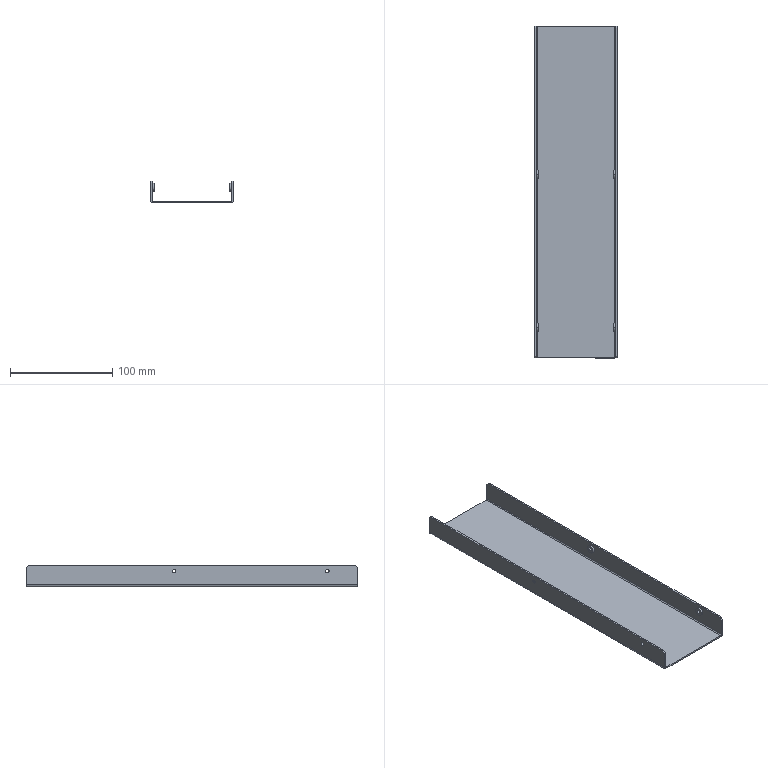Part | SolidWorks | features Chamfer 1, EdgeFlange 1, FlatPattern 1, HoleWzd 1, ICE 1, MirrorPattern 1, SMBaseFlange 1, SheetMetal 1 | 1 solid | 46 faces | box 81 x 325 x 21.5 mm | volume 58526 mm3 | plane 26 | cylinder 20 | commonest cylinder face diameters 3.3 x8 8 x8 2 x2 5 x2
STEP:
#1=CARTESIAN_POINT('',(37.,-132.5,12.35));
#2=VERTEX_POINT('',#1);
#3=CARTESIAN_POINT('',(37.,-132.5,15.65));
#4=VERTEX_POINT('',#3);
#5=CARTESIAN_POINT('',(37.,-132.5,14.));
#6=DIRECTION('',(-1.,0.,0.));
#7=DIRECTION('',(0.,0.,1.));
#8=AXIS2_PLACEMENT_3D('',#5,#6,#7);
#9=CIRCLE('',#8,1.65);
#10=EDGE_CURVE('',#2,#4,#9,.T.);
#11=ORIENTED_EDGE('',*,*,#10,.T.);
#12=CARTESIAN_POINT('',(40.5,-132.5,15.65));
#13=VERTEX_POINT('',#12);
#14=CARTESIAN_POINT('',(40.5,-132.5,15.65));
#15=DIRECTION('',(1.,0.,0.));
#16=VECTOR('',#15,1000.);
#17=LINE('',#14,#16);
#18=EDGE_CURVE('',#4,#13,#17,.T.);
#19=ORIENTED_EDGE('',*,*,#18,.T.);
#20=CARTESIAN_POINT('',(40.5,-132.5,12.35));
#21=VERTEX_POINT('',#20);
#22=CARTESIAN_POINT('',(40.5,-132.5,14.));
#23=DIRECTION('',(1.,0.,0.));
#24=DIRECTION('',(0.,0.,-1.));
#25=AXIS2_PLACEMENT_3D('',#22,#23,#24);
#26=CIRCLE('',#25,1.65);
#27=EDGE_CURVE('',#13,#21,#26,.T.);
#28=ORIENTED_EDGE('',*,*,#27,.T.);
#29=CARTESIAN_POINT('',(40.5,-132.5,12.35));
#30=DIRECTION('',(1.,0.,0.));
#31=VECTOR('',#30,1000.);
#32=LINE('',#29,#31);
#33=EDGE_CURVE('',#2,#21,#32,.T.);
#34=ORIENTED_EDGE('',*,*,#33,.F.);
#35=EDGE_LOOP('',(#11,#19,#28,#34));
#36=FACE_OUTER_BOUND('',#35,.T.);
#37=CARTESIAN_POINT('',(40.5,-132.5,14.));
#38=DIRECTION('',(1.,0.,0.));
#39=DIRECTION('',(0.,0.,-1.));
#40=AXIS2_PLACEMENT_3D('',#37,#38,#39);
#41=CYLINDRICAL_SURFACE('',#40,1.65);
#42=ADVANCED_FACE('',(#36),#41,.F.);
#43=CARTESIAN_POINT('',(37.,17.5,12.35));
#44=VERTEX_POINT('',#43);
#45=CARTESIAN_POINT('',(37.,17.5,15.65));
#46=VERTEX_POINT('',#45);
#47=CARTESIAN_POINT('',(37.,17.5,14.));
#48=DIRECTION('',(-1.,0.,0.));
#49=DIRECTION('',(0.,0.,1.));
#50=AXIS2_PLACEMENT_3D('',#47,#48,#49);
#51=CIRCLE('',#50,1.65);
#52=EDGE_CURVE('',#44,#46,#51,.T.);
#53=ORIENTED_EDGE('',*,*,#52,.T.);
#54=CARTESIAN_POINT('',(40.5,17.5,15.65));
#55=VERTEX_POINT('',#54);
#56=CARTESIAN_POINT('',(40.5,17.5,15.65));
#57=DIRECTION('',(1.,0.,0.));
#58=VECTOR('',#57,1000.);
#59=LINE('',#56,#58);
#60=EDGE_CURVE('',#46,#55,#59,.T.);
#61=ORIENTED_EDGE('',*,*,#60,.T.);
#62=CARTESIAN_POINT('',(40.5,17.5,12.35));
#63=VERTEX_POINT('',#62);
#64=CARTESIAN_POINT('',(40.5,17.5,14.));
#65=DIRECTION('',(1.,0.,0.));
#66=DIRECTION('',(0.,0.,-1.));
#67=AXIS2_PLACEMENT_3D('',#64,#65,#66);
#68=CIRCLE('',#67,1.65);
#69=EDGE_CURVE('',#55,#63,#68,.T.);
#70=ORIENTED_EDGE('',*,*,#69,.T.);
#71=CARTESIAN_POINT('',(40.5,17.5,12.35));
#72=DIRECTION('',(1.,0.,0.));
#73=VECTOR('',#72,1000.);
#74=LINE('',#71,#73);
#75=EDGE_CURVE('',#44,#63,#74,.T.);
#76=ORIENTED_EDGE('',*,*,#75,.F.);
#77=EDGE_LOOP('',(#53,#61,#70,#76));
#78=FACE_OUTER_BOUND('',#77,.T.);
#79=CARTESIAN_POINT('',(40.5,17.5,14.));
#80=DIRECTION('',(1.,0.,0.));
#81=DIRECTION('',(0.,0.,-1.));
#82=AXIS2_PLACEMENT_3D('',#79,#80,#81);
#83=CYLINDRICAL_SURFACE('',#82,1.65);
#84=ADVANCED_FACE('',(#78),#83,.F.);
#85=CARTESIAN_POINT('',(37.,-132.5,10.));
#86=VERTEX_POINT('',#85);
#87=CARTESIAN_POINT('',(37.,-132.5,18.));
#88=VERTEX_POINT('',#87);
#89=CARTESIAN_POINT('',(37.,-132.5,14.));
#90=DIRECTION('',(1.,0.,0.));
#91=DIRECTION('',(0.,0.,-1.));
#92=AXIS2_PLACEMENT_3D('',#89,#90,#91);
#93=CIRCLE('',#92,4.);
#94=EDGE_CURVE('',#86,#88,#93,.T.);
#95=ORIENTED_EDGE('',*,*,#94,.T.);
#96=CARTESIAN_POINT('',(39.,-132.5,18.));
#97=VERTEX_POINT('',#96);
#98=CARTESIAN_POINT('',(37.,-132.5,18.));
#99=DIRECTION('',(1.,0.,0.));
#100=VECTOR('',#99,1000.);
#101=LINE('',#98,#100);
#102=EDGE_CURVE('',#88,#97,#101,.T.);
#103=ORIENTED_EDGE('',*,*,#102,.T.);
#104=CARTESIAN_POINT('',(39.,-132.5,10.));
#105=VERTEX_POINT('',#104);
#106=CARTESIAN_POINT('',(39.,-132.5,14.));
#107=DIRECTION('',(-1.,0.,0.));
#108=DIRECTION('',(0.,0.,1.));
#109=AXIS2_PLACEMENT_3D('',#106,#107,#108);
#110=CIRCLE('',#109,4.);
#111=EDGE_CURVE('',#97,#105,#110,.T.);
#112=ORIENTED_EDGE('',*,*,#111,.T.);
#113=CARTESIAN_POINT('',(37.,-132.5,10.));
#114=DIRECTION('',(1.,0.,0.));
#115=VECTOR('',#114,1000.);
#116=LINE('',#113,#115);
#117=EDGE_CURVE('',#86,#105,#116,.T.);
#118=ORIENTED_EDGE('',*,*,#117,.F.);
#119=EDGE_LOOP('',(#95,#103,#112,#118));
#120=FACE_OUTER_BOUND('',#119,.T.);
#121=CARTESIAN_POINT('',(37.,-132.5,14.));
#122=DIRECTION('',(1.,0.,0.));
#123=DIRECTION('',(0.,0.,-1.));
#124=AXIS2_PLACEMENT_3D('',#121,#122,#123);
#125=CYLINDRICAL_SURFACE('',#124,4.);
#126=ADVANCED_FACE('',(#120),#125,.T.);
#127=CARTESIAN_POINT('',(37.,17.5,10.));
#128=VERTEX_POINT('',#127);
#129=CARTESIAN_POINT('',(37.,17.5,18.));
#130=VERTEX_POINT('',#129);
#131=CARTESIAN_POINT('',(37.,17.5,14.));
#132=DIRECTION('',(1.,0.,0.));
#133=DIRECTION('',(0.,0.,-1.));
#134=AXIS2_PLACEMENT_3D('',#131,#132,#133);
#135=CIRCLE('',#134,4.);
#136=EDGE_CURVE('',#128,#130,#135,.T.);
#137=ORIENTED_EDGE('',*,*,#136,.T.);
#138=CARTESIAN_POINT('',(39.,17.5,18.));
#139=VERTEX_POINT('',#138);
#140=CARTESIAN_POINT('',(37.,17.5,18.));
#141=DIRECTION('',(1.,0.,0.));
#142=VECTOR('',#141,1000.);
#143=LINE('',#140,#142);
#144=EDGE_CURVE('',#130,#139,#143,.T.);
#145=ORIENTED_EDGE('',*,*,#144,.T.);
#146=CARTESIAN_POINT('',(39.,17.5,10.));
#147=VERTEX_POINT('',#146);
#148=CARTESIAN_POINT('',(39.,17.5,14.));
#149=DIRECTION('',(-1.,0.,0.));
#150=DIRECTION('',(0.,0.,1.));
#151=AXIS2_PLACEMENT_3D('',#148,#149,#150);
#152=CIRCLE('',#151,4.);
#153=EDGE_CURVE('',#139,#147,#152,.T.);
#154=ORIENTED_EDGE('',*,*,#153,.T.);
#155=CARTESIAN_POINT('',(37.,17.5,10.));
#156=DIRECTION('',(1.,0.,0.));
#157=VECTOR('',#156,1000.);
#158=LINE('',#155,#157);
#159=EDGE_CURVE('',#128,#147,#158,.T.);
#160=ORIENTED_EDGE('',*,*,#159,.F.);
#161=EDGE_LOOP('',(#137,#145,#154,#160));
#162=FACE_OUTER_BOUND('',#161,.T.);
#163=CARTESIAN_POINT('',(37.,17.5,14.));
#164=DIRECTION('',(1.,0.,0.));
#165=DIRECTION('',(0.,0.,-1.));
#166=AXIS2_PLACEMENT_3D('',#163,#164,#165);
#167=CYLINDRICAL_SURFACE('',#166,4.);
#168=ADVANCED_FACE('',(#162),#167,.T.);
#169=CARTESIAN_POINT('',(-37.,-132.5,15.65));
#170=VERTEX_POINT('',#169);
#171=CARTESIAN_POINT('',(-37.,-132.5,12.35));
#172=VERTEX_POINT('',#171);
#173=CARTESIAN_POINT('',(-37.,-132.5,14.));
#174=DIRECTION('',(1.,0.,0.));
#175=DIRECTION('',(0.,0.,-1.));
#176=AXIS2_PLACEMENT_3D('',#173,#174,#175);
#177=CIRCLE('',#176,1.65);
#178=EDGE_CURVE('',#170,#172,#177,.T.);
#179=ORIENTED_EDGE('',*,*,#178,.T.);
#180=CARTESIAN_POINT('',(-40.5,-132.5,12.35));
#181=VERTEX_POINT('',#180);
#182=CARTESIAN_POINT('',(-40.5,-132.5,12.35));
#183=DIRECTION('',(-1.,0.,0.));
#184=VECTOR('',#183,1000.);
#185=LINE('',#182,#184);
#186=EDGE_CURVE('',#172,#181,#185,.T.);
#187=ORIENTED_EDGE('',*,*,#186,.T.);
#188=CARTESIAN_POINT('',(-40.5,-132.5,15.65));
#189=VERTEX_POINT('',#188);
#190=CARTESIAN_POINT('',(-40.5,-132.5,14.));
#191=DIRECTION('',(-1.,0.,0.));
#192=DIRECTION('',(0.,0.,1.));
#193=AXIS2_PLACEMENT_3D('',#190,#191,#192);
#194=CIRCLE('',#193,1.65);
#195=EDGE_CURVE('',#181,#189,#194,.T.);
#196=ORIENTED_EDGE('',*,*,#195,.T.);
#197=CARTESIAN_POINT('',(-40.5,-132.5,15.65));
#198=DIRECTION('',(-1.,0.,0.));
#199=VECTOR('',#198,1000.);
#200=LINE('',#197,#199);
#201=EDGE_CURVE('',#170,#189,#200,.T.);
#202=ORIENTED_EDGE('',*,*,#201,.F.);
#203=EDGE_LOOP('',(#179,#187,#196,#202));
#204=FACE_OUTER_BOUND('',#203,.T.);
#205=CARTESIAN_POINT('',(-40.5,-132.5,14.));
#206=DIRECTION('',(-1.,0.,0.));
#207=DIRECTION('',(0.,0.,1.));
#208=AXIS2_PLACEMENT_3D('',#205,#206,#207);
#209=CYLINDRICAL_SURFACE('',#208,1.65);
#210=ADVANCED_FACE('',(#204),#209,.F.);
#211=CARTESIAN_POINT('',(-37.,17.5,15.65));
#212=VERTEX_POINT('',#211);
#213=CARTESIAN_POINT('',(-37.,17.5,12.35));
#214=VERTEX_POINT('',#213);
#215=CARTESIAN_POINT('',(-37.,17.5,14.));
#216=DIRECTION('',(1.,0.,0.));
#217=DIRECTION('',(0.,0.,-1.));
#218=AXIS2_PLACEMENT_3D('',#215,#216,#217);
#219=CIRCLE('',#218,1.65);
#220=EDGE_CURVE('',#212,#214,#219,.T.);
#221=ORIENTED_EDGE('',*,*,#220,.T.);
#222=CARTESIAN_POINT('',(-40.5,17.5,12.35));
#223=VERTEX_POINT('',#222);
#224=CARTESIAN_POINT('',(-40.5,17.5,12.35));
#225=DIRECTION('',(-1.,0.,0.));
#226=VECTOR('',#225,1000.);
#227=LINE('',#224,#226);
#228=EDGE_CURVE('',#214,#223,#227,.T.);
#229=ORIENTED_EDGE('',*,*,#228,.T.);
#230=CARTESIAN_POINT('',(-40.5,17.5,15.65));
#231=VERTEX_POINT('',#230);
#232=CARTESIAN_POINT('',(-40.5,17.5,14.));
#233=DIRECTION('',(-1.,0.,0.));
#234=DIRECTION('',(0.,0.,1.));
#235=AXIS2_PLACEMENT_3D('',#232,#233,#234);
#236=CIRCLE('',#235,1.65);
#237=EDGE_CURVE('',#223,#231,#236,.T.);
#238=ORIENTED_EDGE('',*,*,#237,.T.);
#239=CARTESIAN_POINT('',(-40.5,17.5,15.65));
#240=DIRECTION('',(-1.,0.,0.));
#241=VECTOR('',#240,1000.);
#242=LINE('',#239,#241);
#243=EDGE_CURVE('',#212,#231,#242,.T.);
#244=ORIENTED_EDGE('',*,*,#243,.F.);
#245=EDGE_LOOP('',(#221,#229,#238,#244));
#246=FACE_OUTER_BOUND('',#245,.T.);
#247=CARTESIAN_POINT('',(-40.5,17.5,14.));
#248=DIRECTION('',(-1.,0.,0.));
#249=DIRECTION('',(0.,0.,1.));
#250=AXIS2_PLACEMENT_3D('',#247,#248,#249);
#251=CYLINDRICAL_SURFACE('',#250,1.65);
#252=ADVANCED_FACE('',(#246),#251,.F.);
#253=CARTESIAN_POINT('',(-37.,-132.5,10.));
#254=VERTEX_POINT('',#253);
#255=CARTESIAN_POINT('',(-37.,-132.5,18.));
#256=VERTEX_POINT('',#255);
#257=CARTESIAN_POINT('',(-37.,-132.5,14.));
#258=DIRECTION('',(1.,0.,0.));
#259=DIRECTION('',(0.,0.,-1.));
#260=AXIS2_PLACEMENT_3D('',#257,#258,#259);
#261=CIRCLE('',#260,4.);
#262=EDGE_CURVE('',#254,#256,#261,.T.);
#263=ORIENTED_EDGE('',*,*,#262,.F.);
#264=CARTESIAN_POINT('',(-39.,-132.5,10.));
#265=VERTEX_POINT('',#264);
#266=CARTESIAN_POINT('',(-37.,-132.5,10.));
#267=DIRECTION('',(-1.,0.,0.));
#268=VECTOR('',#267,1000.);
#269=LINE('',#266,#268);
#270=EDGE_CURVE('',#254,#265,#269,.T.);
#271=ORIENTED_EDGE('',*,*,#270,.T.);
#272=CARTESIAN_POINT('',(-39.,-132.5,18.));
#273=VERTEX_POINT('',#272);
#274=CARTESIAN_POINT('',(-39.,-132.5,14.));
#275=DIRECTION('',(1.,0.,0.));
#276=DIRECTION('',(0.,0.,-1.));
#277=AXIS2_PLACEMENT_3D('',#274,#275,#276);
#278=CIRCLE('',#277,4.);
#279=EDGE_CURVE('',#265,#273,#278,.T.);
#280=ORIENTED_EDGE('',*,*,#279,.T.);
#281=CARTESIAN_POINT('',(-37.,-132.5,18.));
#282=DIRECTION('',(-1.,0.,0.));
#283=VECTOR('',#282,1000.);
#284=LINE('',#281,#283);
#285=EDGE_CURVE('',#256,#273,#284,.T.);
#286=ORIENTED_EDGE('',*,*,#285,.F.);
#287=EDGE_LOOP('',(#263,#271,#280,#286));
#288=FACE_OUTER_BOUND('',#287,.T.);
#289=CARTESIAN_POINT('',(-37.,-132.5,14.));
#290=DIRECTION('',(-1.,0.,0.));
#291=DIRECTION('',(0.,0.,1.));
#292=AXIS2_PLACEMENT_3D('',#289,#290,#291);
#293=CYLINDRICAL_SURFACE('',#292,4.);
#294=ADVANCED_FACE('',(#288),#293,.T.);
#295=CARTESIAN_POINT('',(-37.,17.5,10.));
#296=VERTEX_POINT('',#295);
#297=CARTESIAN_POINT('',(-37.,17.5,18.));
#298=VERTEX_POINT('',#297);
#299=CARTESIAN_POINT('',(-37.,17.5,14.));
#300=DIRECTION('',(1.,0.,0.));
#301=DIRECTION('',(0.,0.,-1.));
#302=AXIS2_PLACEMENT_3D('',#299,#300,#301);
#303=CIRCLE('',#302,4.);
#304=EDGE_CURVE('',#296,#298,#303,.T.);
#305=ORIENTED_EDGE('',*,*,#304,.F.);
#306=CARTESIAN_POINT('',(-39.,17.5,10.));
#307=VERTEX_POINT('',#306);
#308=CARTESIAN_POINT('',(-37.,17.5,10.));
#309=DIRECTION('',(-1.,0.,0.));
#310=VECTOR('',#309,1000.);
#311=LINE('',#308,#310);
#312=EDGE_CURVE('',#296,#307,#311,.T.);
#313=ORIENTED_EDGE('',*,*,#312,.T.);
#314=CARTESIAN_POINT('',(-39.,17.5,18.));
#315=VERTEX_POINT('',#314);
#316=CARTESIAN_POINT('',(-39.,17.5,14.));
#317=DIRECTION('',(1.,0.,0.));
#318=DIRECTION('',(0.,0.,-1.));
#319=AXIS2_PLACEMENT_3D('',#316,#317,#318);
#320=CIRCLE('',#319,4.);
#321=EDGE_CURVE('',#307,#315,#320,.T.);
#322=ORIENTED_EDGE('',*,*,#321,.T.);
#323=CARTESIAN_POINT('',(-37.,17.5,18.));
#324=DIRECTION('',(-1.,0.,0.));
#325=VECTOR('',#324,1000.);
#326=LINE('',#323,#325);
#327=EDGE_CURVE('',#298,#315,#326,.T.);
#328=ORIENTED_EDGE('',*,*,#327,.F.);
#329=EDGE_LOOP('',(#305,#313,#322,#328));
#330=FACE_OUTER_BOUND('',#329,.T.);
#331=CARTESIAN_POINT('',(-37.,17.5,14.));
#332=DIRECTION('',(-1.,0.,0.));
#333=DIRECTION('',(0.,0.,1.));
#334=AXIS2_PLACEMENT_3D('',#331,#332,#333);
#335=CYLINDRICAL_SURFACE('',#334,4.);
#336=ADVANCED_FACE('',(#330),#335,.T.);
#337=CARTESIAN_POINT('',(40.5,160.5,20.));
#338=VERTEX_POINT('',#337);
#339=CARTESIAN_POINT('',(40.5,-160.5,20.));
#340=VERTEX_POINT('',#339);
#341=CARTESIAN_POINT('',(40.5,-162.5,20.));
#342=DIRECTION('',(0.,-1.,0.));
#343=VECTOR('',#342,1000.);
#344=LINE('',#341,#343);
#345=EDGE_CURVE('',#338,#340,#344,.T.);
#346=ORIENTED_EDGE('',*,*,#345,.T.);
#347=CARTESIAN_POINT('',(40.5,-162.5,18.));
#348=VERTEX_POINT('',#347);
#349=CARTESIAN_POINT('',(40.5,-162.5,18.));
#350=DIRECTION('',(0.,-0.7071,-0.7071));
#351=VECTOR('',#350,1000.);
#352=LINE('',#349,#351);
#353=EDGE_CURVE('',#340,#348,#352,.T.);
#354=ORIENTED_EDGE('',*,*,#353,.T.);
#355=CARTESIAN_POINT('',(40.5,-162.5,1.));
#356=VERTEX_POINT('',#355);
#357=CARTESIAN_POINT('',(40.5,-162.5,0.));
#358=DIRECTION('',(0.,0.,-1.));
#359=VECTOR('',#358,1000.);
#360=LINE('',#357,#359);
#361=EDGE_CURVE('',#348,#356,#360,.T.);
#362=ORIENTED_EDGE('',*,*,#361,.T.);
#363=CARTESIAN_POINT('',(40.5,162.5,1.));
#364=VERTEX_POINT('',#363);
#365=CARTESIAN_POINT('',(40.5,0.,1.));
#366=DIRECTION('',(0.,-1.,0.));
#367=VECTOR('',#366,1000.);
#368=LINE('',#365,#367);
#369=EDGE_CURVE('',#364,#356,#368,.T.);
#370=ORIENTED_EDGE('',*,*,#369,.F.);
#371=CARTESIAN_POINT('',(40.5,162.5,18.));
#372=VERTEX_POINT('',#371);
#373=CARTESIAN_POINT('',(40.5,162.5,20.));
#374=DIRECTION('',(0.,0.,1.));
#375=VECTOR('',#374,1000.);
#376=LINE('',#373,#375);
#377=EDGE_CURVE('',#364,#372,#376,.T.);
#378=ORIENTED_EDGE('',*,*,#377,.T.);
#379=CARTESIAN_POINT('',(40.5,160.5,20.));
#380=DIRECTION('',(0.,-0.7071,0.7071));
#381=VECTOR('',#380,1000.);
#382=LINE('',#379,#381);
#383=EDGE_CURVE('',#372,#338,#382,.T.);
#384=ORIENTED_EDGE('',*,*,#383,.T.);
#385=EDGE_LOOP('',(#346,#354,#362,#370,#378,#384));
#386=FACE_OUTER_BOUND('',#385,.T.);
#387=CARTESIAN_POINT('',(40.5,17.5,14.));
#388=DIRECTION('',(1.,0.,0.));
#389=DIRECTION('',(0.,0.,-1.));
#390=AXIS2_PLACEMENT_3D('',#387,#388,#389);
#391=CIRCLE('',#390,1.65);
#392=EDGE_CURVE('',#63,#55,#391,.T.);
#393=ORIENTED_EDGE('',*,*,#392,.F.);
#394=ORIENTED_EDGE('',*,*,#69,.F.);
#395=EDGE_LOOP('',(#393,#394));
#396=FACE_BOUND('',#395,.T.);
#397=CARTESIAN_POINT('',(40.5,-132.5,14.));
#398=DIRECTION('',(1.,0.,0.));
#399=DIRECTION('',(0.,0.,-1.));
#400=AXIS2_PLACEMENT_3D('',#397,#398,#399);
#401=CIRCLE('',#400,1.65);
#402=EDGE_CURVE('',#21,#13,#401,.T.);
#403=ORIENTED_EDGE('',*,*,#402,.F.);
#404=ORIENTED_EDGE('',*,*,#27,.F.);
#405=EDGE_LOOP('',(#403,#404));
#406=FACE_BOUND('',#405,.T.);
#407=CARTESIAN_POINT('',(40.5,0.,0.));
#408=DIRECTION('',(-1.,0.,0.));
#409=DIRECTION('',(0.,0.,1.));
#410=AXIS2_PLACEMENT_3D('',#407,#408,#409);
#411=PLANE('',#410);
#412=ADVANCED_FACE('',(#386,#396,#406),#411,.F.);
#413=CARTESIAN_POINT('',(-39.,17.5,14.));
#414=DIRECTION('',(1.,0.,0.));
#415=DIRECTION('',(0.,0.,-1.));
#416=AXIS2_PLACEMENT_3D('',#413,#414,#415);
#417=CIRCLE('',#416,4.);
#418=EDGE_CURVE('',#315,#307,#417,.T.);
#419=ORIENTED_EDGE('',*,*,#418,.F.);
#420=ORIENTED_EDGE('',*,*,#321,.F.);
#421=EDGE_LOOP('',(#419,#420));
#422=FACE_BOUND('',#421,.T.);
#423=CARTESIAN_POINT('',(-39.,-160.5,20.));
#424=VERTEX_POINT('',#423);
#425=CARTESIAN_POINT('',(-39.,160.5,20.));
#426=VERTEX_POINT('',#425);
#427=CARTESIAN_POINT('',(-39.,162.5,20.));
#428=DIRECTION('',(0.,1.,0.));
#429=VECTOR('',#428,1000.);
#430=LINE('',#427,#429);
#431=EDGE_CURVE('',#424,#426,#430,.T.);
#432=ORIENTED_EDGE('',*,*,#431,.F.);
#433=CARTESIAN_POINT('',(-39.,-162.5,18.));
#434=VERTEX_POINT('',#433);
#435=CARTESIAN_POINT('',(-39.,-90.25,90.25));
#436=DIRECTION('',(0.,-0.7071,-0.7071));
#437=VECTOR('',#436,1000.);
#438=LINE('',#435,#437);
#439=EDGE_CURVE('',#424,#434,#438,.T.);
#440=ORIENTED_EDGE('',*,*,#439,.T.);
#441=CARTESIAN_POINT('',(-39.,-162.5,1.));
#442=VERTEX_POINT('',#441);
#443=CARTESIAN_POINT('',(-39.,-162.5,20.));
#444=DIRECTION('',(0.,0.,1.));
#445=VECTOR('',#444,1000.);
#446=LINE('',#443,#445);
#447=EDGE_CURVE('',#442,#434,#446,.T.);
#448=ORIENTED_EDGE('',*,*,#447,.F.);
#449=CARTESIAN_POINT('',(-39.,162.5,1.));
#450=VERTEX_POINT('',#449);
#451=CARTESIAN_POINT('',(-39.,162.5,1.));
#452=DIRECTION('',(0.,-1.,0.));
#453=VECTOR('',#452,1000.);
#454=LINE('',#451,#453);
#455=EDGE_CURVE('',#450,#442,#454,.T.);
#456=ORIENTED_EDGE('',*,*,#455,.F.);
#457=CARTESIAN_POINT('',(-39.,162.5,18.));
#458=VERTEX_POINT('',#457);
#459=CARTESIAN_POINT('',(-39.,162.5,0.));
#460=DIRECTION('',(0.,0.,-1.));
#461=VECTOR('',#460,1000.);
#462=LINE('',#459,#461);
#463=EDGE_CURVE('',#458,#450,#462,.T.);
#464=ORIENTED_EDGE('',*,*,#463,.F.);
#465=CARTESIAN_POINT('',(-39.,90.25,90.25));
#466=DIRECTION('',(0.,-0.7071,0.7071));
#467=VECTOR('',#466,1000.);
#468=LINE('',#465,#467);
#469=EDGE_CURVE('',#458,#426,#468,.T.);
#470=ORIENTED_EDGE('',*,*,#469,.T.);
#471=EDGE_LOOP('',(#432,#440,#448,#456,#464,#470));
#472=FACE_OUTER_BOUND('',#471,.T.);
#473=CARTESIAN_POINT('',(-39.,-132.5,14.));
#474=DIRECTION('',(1.,0.,0.));
#475=DIRECTION('',(0.,0.,-1.));
#476=AXIS2_PLACEMENT_3D('',#473,#474,#475);
#477=CIRCLE('',#476,4.);
#478=EDGE_CURVE('',#273,#265,#477,.T.);
#479=ORIENTED_EDGE('',*,*,#478,.F.);
#480=ORIENTED_EDGE('',*,*,#279,.F.);
#481=EDGE_LOOP('',(#479,#480));
#482=FACE_BOUND('',#481,.T.);
#483=CARTESIAN_POINT('',(-39.,0.,0.));
#484=DIRECTION('',(1.,0.,0.));
#485=DIRECTION('',(0.,0.,-1.));
#486=AXIS2_PLACEMENT_3D('',#483,#484,#485);
#487=PLANE('',#486);
#488=ADVANCED_FACE('',(#422,#472,#482),#487,.T.);
#489=CARTESIAN_POINT('',(38.,162.5,-1.5));
#490=VERTEX_POINT('',#489);
#491=CARTESIAN_POINT('',(38.,-162.5,-1.5));
#492=VERTEX_POINT('',#491);
#493=CARTESIAN_POINT('',(38.,162.5,-1.5));
#494=DIRECTION('',(0.,-1.,0.));
#495=VECTOR('',#494,1000.);
#496=LINE('',#493,#495);
#497=EDGE_CURVE('',#490,#492,#496,.T.);
#498=ORIENTED_EDGE('',*,*,#497,.T.);
#499=CARTESIAN_POINT('',(-38.,-162.5,-1.5));
#500=VERTEX_POINT('',#499);
#501=CARTESIAN_POINT('',(-39.,-162.5,-1.5));
#502=DIRECTION('',(1.,0.,0.));
#503=VECTOR('',#502,1000.);
#504=LINE('',#501,#503);
#505=EDGE_CURVE('',#500,#492,#504,.T.);
#506=ORIENTED_EDGE('',*,*,#505,.F.);
#507=CARTESIAN_POINT('',(-38.,162.5,-1.5));
#508=VERTEX_POINT('',#507);
#509=CARTESIAN_POINT('',(-38.,-162.5,-1.5));
#510=DIRECTION('',(0.,1.,0.));
#511=VECTOR('',#510,1000.);
#512=LINE('',#509,#511);
#513=EDGE_CURVE('',#500,#508,#512,.T.);
#514=ORIENTED_EDGE('',*,*,#513,.T.);
#515=CARTESIAN_POINT('',(-39.,162.5,-1.5));
#516=DIRECTION('',(-1.,0.,0.));
#517=VECTOR('',#516,1000.);
#518=LINE('',#515,#517);
#519=EDGE_CURVE('',#490,#508,#518,.T.);
#520=ORIENTED_EDGE('',*,*,#519,.F.);
#521=EDGE_LOOP('',(#498,#506,#514,#520));
#522=FACE_OUTER_BOUND('',#521,.T.);
#523=CARTESIAN_POINT('',(0.,0.,-1.5));
#524=DIRECTION('',(0.,0.,1.));
#525=DIRECTION('',(1.,0.,0.));
#526=AXIS2_PLACEMENT_3D('',#523,#524,#525);
#527=PLANE('',#526);
#528=ADVANCED_FACE('',(#522),#527,.F.);
#529=CARTESIAN_POINT('',(-38.,-162.5,0.));
#530=VERTEX_POINT('',#529);
#531=CARTESIAN_POINT('',(38.,-162.5,0.));
#532=VERTEX_POINT('',#531);
#533=CARTESIAN_POINT('',(-39.,-162.5,0.));
#534=DIRECTION('',(1.,0.,0.));
#535=VECTOR('',#534,1000.);
#536=LINE('',#533,#535);
#537=EDGE_CURVE('',#530,#532,#536,.T.);
#538=ORIENTED_EDGE('',*,*,#537,.T.);
#539=CARTESIAN_POINT('',(38.,162.5,0.));
#540=VERTEX_POINT('',#539);
#541=CARTESIAN_POINT('',(38.,162.5,0.));
#542=DIRECTION('',(0.,-1.,0.));
#543=VECTOR('',#542,1000.);
#544=LINE('',#541,#543);
#545=EDGE_CURVE('',#540,#532,#544,.T.);
#546=ORIENTED_EDGE('',*,*,#545,.F.);
#547=CARTESIAN_POINT('',(-38.,162.5,0.));
#548=VERTEX_POINT('',#547);
#549=CARTESIAN_POINT('',(-39.,162.5,0.));
#550=DIRECTION('',(-1.,0.,0.));
#551=VECTOR('',#550,1000.);
#552=LINE('',#549,#551);
#553=EDGE_CURVE('',#540,#548,#552,.T.);
#554=ORIENTED_EDGE('',*,*,#553,.T.);
#555=CARTESIAN_POINT('',(-38.,-162.5,0.));
#556=DIRECTION('',(0.,1.,0.));
#557=VECTOR('',#556,1000.);
#558=LINE('',#555,#557);
#559=EDGE_CURVE('',#530,#548,#558,.T.);
#560=ORIENTED_EDGE('',*,*,#559,.F.);
#561=EDGE_LOOP('',(#538,#546,#554,#560));
#562=FACE_OUTER_BOUND('',#561,.T.);
#563=CARTESIAN_POINT('',(0.,0.,0.));
#564=DIRECTION('',(0.,0.,1.));
#565=DIRECTION('',(1.,0.,0.));
#566=AXIS2_PLACEMENT_3D('',#563,#564,#565);
#567=PLANE('',#566);
#568=ADVANCED_FACE('',(#562),#567,.T.);
#569=ORIENTED_EDGE('',*,*,#553,.F.);
#570=CARTESIAN_POINT('',(38.,162.5,0.));
#571=DIRECTION('',(0.,0.,-1.));
#572=VECTOR('',#571,1000.);
#573=LINE('',#570,#572);
#574=EDGE_CURVE('',#540,#490,#573,.T.);
#575=ORIENTED_EDGE('',*,*,#574,.T.);
#576=ORIENTED_EDGE('',*,*,#519,.T.);
#577=CARTESIAN_POINT('',(-38.,162.5,0.));
#578=DIRECTION('',(0.,0.,-1.));
#579=VECTOR('',#578,1000.);
#580=LINE('',#577,#579);
#581=EDGE_CURVE('',#548,#508,#580,.T.);
#582=ORIENTED_EDGE('',*,*,#581,.F.);
#583=EDGE_LOOP('',(#569,#575,#576,#582));
#584=FACE_OUTER_BOUND('',#583,.T.);
#585=CARTESIAN_POINT('',(-39.,162.5,-1.5));
#586=DIRECTION('',(0.,1.,0.));
#587=DIRECTION('',(0.,0.,1.));
#588=AXIS2_PLACEMENT_3D('',#585,#586,#587);
#589=PLANE('',#588);
#590=ADVANCED_FACE('',(#584),#589,.T.);
#591=CARTESIAN_POINT('',(38.,-162.5,0.));
#592=DIRECTION('',(0.,0.,-1.));
#593=VECTOR('',#592,1000.);
#594=LINE('',#591,#593);
#595=EDGE_CURVE('',#532,#492,#594,.T.);
#596=ORIENTED_EDGE('',*,*,#595,.F.);
#597=ORIENTED_EDGE('',*,*,#537,.F.);
#598=CARTESIAN_POINT('',(-38.,-162.5,0.));
#599=DIRECTION('',(0.,0.,-1.));
#600=VECTOR('',#599,1000.);
#601=LINE('',#598,#600);
#602=EDGE_CURVE('',#530,#500,#601,.T.);
#603=ORIENTED_EDGE('',*,*,#602,.T.);
#604=ORIENTED_EDGE('',*,*,#505,.T.);
#605=EDGE_LOOP('',(#596,#597,#603,#604));
#606=FACE_OUTER_BOUND('',#605,.T.);
#607=CARTESIAN_POINT('',(-39.,-162.5,-1.5));
#608=DIRECTION('',(0.,-1.,0.));
#609=DIRECTION('',(0.,0.,-1.));
#610=AXIS2_PLACEMENT_3D('',#607,#608,#609);
#611=PLANE('',#610);
#612=ADVANCED_FACE('',(#606),#611,.T.);
#613=CARTESIAN_POINT('',(-40.5,162.5,1.));
#614=VERTEX_POINT('',#613);
#615=CARTESIAN_POINT('',(-39.,162.5,1.));
#616=DIRECTION('',(-1.,0.,0.));
#617=VECTOR('',#616,1000.);
#618=LINE('',#615,#617);
#619=EDGE_CURVE('',#450,#614,#618,.T.);
#620=ORIENTED_EDGE('',*,*,#619,.F.);
#621=CARTESIAN_POINT('',(-38.,162.5,1.));
#622=DIRECTION('',(0.,1.,0.));
#623=DIRECTION('',(0.,0.,-1.));
#624=AXIS2_PLACEMENT_3D('',#621,#622,#623);
#625=CIRCLE('',#624,1.);
#626=EDGE_CURVE('',#548,#450,#625,.T.);
#627=ORIENTED_EDGE('',*,*,#626,.F.);
#628=ORIENTED_EDGE('',*,*,#581,.T.);
#629=CARTESIAN_POINT('',(-38.,162.5,1.));
#630=DIRECTION('',(0.,1.,0.));
#631=DIRECTION('',(0.,0.,-1.));
#632=AXIS2_PLACEMENT_3D('',#629,#630,#631);
#633=CIRCLE('',#632,2.5);
#634=EDGE_CURVE('',#508,#614,#633,.T.);
#635=ORIENTED_EDGE('',*,*,#634,.T.);
#636=EDGE_LOOP('',(#620,#627,#628,#635));
#637=FACE_OUTER_BOUND('',#636,.T.);
#638=CARTESIAN_POINT('',(-38.,162.5,1.));
#639=DIRECTION('',(0.,1.,0.));
#640=DIRECTION('',(0.,0.,1.));
#641=AXIS2_PLACEMENT_3D('',#638,#639,#640);
#642=PLANE('',#641);
#643=ADVANCED_FACE('',(#637),#642,.T.);
#644=CARTESIAN_POINT('',(-38.,-162.5,1.));
#645=DIRECTION('',(0.,-1.,0.));
#646=DIRECTION('',(0.,0.,-1.));
#647=AXIS2_PLACEMENT_3D('',#644,#645,#646);
#648=CIRCLE('',#647,1.);
#649=EDGE_CURVE('',#442,#530,#648,.T.);
#650=ORIENTED_EDGE('',*,*,#649,.F.);
#651=CARTESIAN_POINT('',(-40.5,-162.5,1.));
#652=VERTEX_POINT('',#651);
#653=CARTESIAN_POINT('',(-39.,-162.5,1.));
#654=DIRECTION('',(-1.,0.,0.));
#655=VECTOR('',#654,1000.);
#656=LINE('',#653,#655);
#657=EDGE_CURVE('',#442,#652,#656,.T.);
#658=ORIENTED_EDGE('',*,*,#657,.T.);
#659=CARTESIAN_POINT('',(-38.,-162.5,1.));
#660=DIRECTION('',(0.,-1.,0.));
#661=DIRECTION('',(0.,0.,-1.));
#662=AXIS2_PLACEMENT_3D('',#659,#660,#661);
#663=CIRCLE('',#662,2.5);
#664=EDGE_CURVE('',#652,#500,#663,.T.);
#665=ORIENTED_EDGE('',*,*,#664,.T.);
#666=ORIENTED_EDGE('',*,*,#602,.F.);
#667=EDGE_LOOP('',(#650,#658,#665,#666));
#668=FACE_OUTER_BOUND('',#667,.T.);
#669=CARTESIAN_POINT('',(-38.,-162.5,1.));
#670=DIRECTION('',(0.,1.,0.));
#671=DIRECTION('',(0.,0.,1.));
#672=AXIS2_PLACEMENT_3D('',#669,#670,#671);
#673=PLANE('',#672);
#674=ADVANCED_FACE('',(#668),#673,.F.);
#675=ORIENTED_EDGE('',*,*,#513,.F.);
#676=ORIENTED_EDGE('',*,*,#664,.F.);
#677=CARTESIAN_POINT('',(-40.5,0.,1.));
#678=DIRECTION('',(0.,1.,0.));
#679=VECTOR('',#678,1000.);
#680=LINE('',#677,#679);
#681=EDGE_CURVE('',#652,#614,#680,.T.);
#682=ORIENTED_EDGE('',*,*,#681,.T.);
#683=ORIENTED_EDGE('',*,*,#634,.F.);
#684=EDGE_LOOP('',(#675,#676,#682,#683));
#685=FACE_OUTER_BOUND('',#684,.T.);
#686=CARTESIAN_POINT('',(-38.,-162.5,1.));
#687=DIRECTION('',(0.,-1.,0.));
#688=DIRECTION('',(-1.,0.,0.));
#689=AXIS2_PLACEMENT_3D('',#686,#687,#688);
#690=CYLINDRICAL_SURFACE('',#689,2.5);
#691=ADVANCED_FACE('',(#685),#690,.T.);
#692=ORIENTED_EDGE('',*,*,#559,.T.);
#693=ORIENTED_EDGE('',*,*,#626,.T.);
#694=ORIENTED_EDGE('',*,*,#455,.T.);
#695=ORIENTED_EDGE('',*,*,#649,.T.);
#696=EDGE_LOOP('',(#692,#693,#694,#695));
#697=FACE_OUTER_BOUND('',#696,.T.);
#698=CARTESIAN_POINT('',(-38.,-162.5,1.));
#699=DIRECTION('',(0.,-1.,0.));
#700=DIRECTION('',(-1.,0.,0.));
#701=AXIS2_PLACEMENT_3D('',#698,#699,#700);
#702=CYLINDRICAL_SURFACE('',#701,1.);
#703=ADVANCED_FACE('',(#697),#702,.F.);
#704=ORIENTED_EDGE('',*,*,#447,.T.);
#705=CARTESIAN_POINT('',(-40.5,-162.5,18.));
#706=VERTEX_POINT('',#705);
#707=CARTESIAN_POINT('',(-40.5,-162.5,18.));
#708=DIRECTION('',(-1.,0.,0.));
#709=VECTOR('',#708,1000.);
#710=LINE('',#707,#709);
#711=EDGE_CURVE('',#434,#706,#710,.T.);
#712=ORIENTED_EDGE('',*,*,#711,.T.);
#713=CARTESIAN_POINT('',(-40.5,-162.5,20.));
#714=DIRECTION('',(0.,0.,1.));
#715=VECTOR('',#714,1000.);
#716=LINE('',#713,#715);
#717=EDGE_CURVE('',#652,#706,#716,.T.);
#718=ORIENTED_EDGE('',*,*,#717,.F.);
#719=ORIENTED_EDGE('',*,*,#657,.F.);
#720=EDGE_LOOP('',(#704,#712,#718,#719));
#721=FACE_OUTER_BOUND('',#720,.T.);
#722=CARTESIAN_POINT('',(-40.5,-162.5,20.));
#723=DIRECTION('',(0.,1.,0.));
#724=DIRECTION('',(-1.,0.,0.));
#725=AXIS2_PLACEMENT_3D('',#722,#723,#724);
#726=PLANE('',#725);
#727=ADVANCED_FACE('',(#721),#726,.F.);
#728=CARTESIAN_POINT('',(-40.5,162.5,18.));
#729=VERTEX_POINT('',#728);
#730=CARTESIAN_POINT('',(-40.5,162.5,0.));
#731=DIRECTION('',(0.,0.,-1.));
#732=VECTOR('',#731,1000.);
#733=LINE('',#730,#732);
#734=EDGE_CURVE('',#729,#614,#733,.T.);
#735=ORIENTED_EDGE('',*,*,#734,.F.);
#736=CARTESIAN_POINT('',(-40.5,162.5,18.));
#737=DIRECTION('',(1.,0.,0.));
#738=VECTOR('',#737,1000.);
#739=LINE('',#736,#738);
#740=EDGE_CURVE('',#729,#458,#739,.T.);
#741=ORIENTED_EDGE('',*,*,#740,.T.);
#742=ORIENTED_EDGE('',*,*,#463,.T.);
#743=ORIENTED_EDGE('',*,*,#619,.T.);
#744=EDGE_LOOP('',(#735,#741,#742,#743));
#745=FACE_OUTER_BOUND('',#744,.T.);
#746=CARTESIAN_POINT('',(-40.5,162.5,0.));
#747=DIRECTION('',(0.,-1.,0.));
#748=DIRECTION('',(1.,0.,0.));
#749=AXIS2_PLACEMENT_3D('',#746,#747,#748);
#750=PLANE('',#749);
#751=ADVANCED_FACE('',(#745),#750,.F.);
#752=CARTESIAN_POINT('',(-40.5,-132.5,14.));
#753=DIRECTION('',(-1.,0.,0.));
#754=DIRECTION('',(0.,0.,1.));
#755=AXIS2_PLACEMENT_3D('',#752,#753,#754);
#756=CIRCLE('',#755,1.65);
#757=EDGE_CURVE('',#189,#181,#756,.T.);
#758=ORIENTED_EDGE('',*,*,#757,.F.);
#759=ORIENTED_EDGE('',*,*,#195,.F.);
#760=EDGE_LOOP('',(#758,#759));
#761=FACE_BOUND('',#760,.T.);
#762=CARTESIAN_POINT('',(-40.5,17.5,14.));
#763=DIRECTION('',(-1.,0.,0.));
#764=DIRECTION('',(0.,0.,1.));
#765=AXIS2_PLACEMENT_3D('',#762,#763,#764);
#766=CIRCLE('',#765,1.65);
#767=EDGE_CURVE('',#231,#223,#766,.T.);
#768=ORIENTED_EDGE('',*,*,#767,.F.);
#769=ORIENTED_EDGE('',*,*,#237,.F.);
#770=EDGE_LOOP('',(#768,#769));
#771=FACE_BOUND('',#770,.T.);
#772=ORIENTED_EDGE('',*,*,#717,.T.);
#773=CARTESIAN_POINT('',(-40.5,-160.5,20.));
#774=VERTEX_POINT('',#773);
#775=CARTESIAN_POINT('',(-40.5,-160.5,20.));
#776=DIRECTION('',(0.,0.7071,0.7071));
#777=VECTOR('',#776,1000.);
#778=LINE('',#775,#777);
#779=EDGE_CURVE('',#706,#774,#778,.T.);
#780=ORIENTED_EDGE('',*,*,#779,.T.);
#781=CARTESIAN_POINT('',(-40.5,160.5,20.));
#782=VERTEX_POINT('',#781);
#783=CARTESIAN_POINT('',(-40.5,162.5,20.));
#784=DIRECTION('',(0.,1.,0.));
#785=VECTOR('',#784,1000.);
#786=LINE('',#783,#785);
#787=EDGE_CURVE('',#774,#782,#786,.T.);
#788=ORIENTED_EDGE('',*,*,#787,.T.);
#789=CARTESIAN_POINT('',(-40.5,162.5,18.));
#790=DIRECTION('',(0.,0.7071,-0.7071));
#791=VECTOR('',#790,1000.);
#792=LINE('',#789,#791);
#793=EDGE_CURVE('',#782,#729,#792,.T.);
#794=ORIENTED_EDGE('',*,*,#793,.T.);
#795=ORIENTED_EDGE('',*,*,#734,.T.);
#796=ORIENTED_EDGE('',*,*,#681,.F.);
#797=EDGE_LOOP('',(#772,#780,#788,#794,#795,#796));
#798=FACE_OUTER_BOUND('',#797,.T.);
#799=CARTESIAN_POINT('',(-40.5,0.,0.));
#800=DIRECTION('',(1.,0.,0.));
#801=DIRECTION('',(0.,0.,-1.));
#802=AXIS2_PLACEMENT_3D('',#799,#800,#801);
#803=PLANE('',#802);
#804=ADVANCED_FACE('',(#761,#771,#798),#803,.F.);
#805=ORIENTED_EDGE('',*,*,#787,.F.);
#806=CARTESIAN_POINT('',(-40.5,-160.5,20.));
#807=DIRECTION('',(1.,0.,0.));
#808=VECTOR('',#807,1000.);
#809=LINE('',#806,#808);
#810=EDGE_CURVE('',#774,#424,#809,.T.);
#811=ORIENTED_EDGE('',*,*,#810,.T.);
#812=ORIENTED_EDGE('',*,*,#431,.T.);
#813=CARTESIAN_POINT('',(-40.5,160.5,20.));
#814=DIRECTION('',(-1.,0.,0.));
#815=VECTOR('',#814,1000.);
#816=LINE('',#813,#815);
#817=EDGE_CURVE('',#426,#782,#816,.T.);
#818=ORIENTED_EDGE('',*,*,#817,.T.);
#819=EDGE_LOOP('',(#805,#811,#812,#818));
#820=FACE_OUTER_BOUND('',#819,.T.);
#821=CARTESIAN_POINT('',(-40.5,162.5,20.));
#822=DIRECTION('',(0.,0.,-1.));
#823=DIRECTION('',(-1.,0.,0.));
#824=AXIS2_PLACEMENT_3D('',#821,#822,#823);
#825=PLANE('',#824);
#826=ADVANCED_FACE('',(#820),#825,.F.);
#827=CARTESIAN_POINT('',(39.,-162.5,1.));
#828=VERTEX_POINT('',#827);
#829=CARTESIAN_POINT('',(39.,-162.5,1.));
#830=DIRECTION('',(1.,0.,0.));
#831=VECTOR('',#830,1000.);
#832=LINE('',#829,#831);
#833=EDGE_CURVE('',#828,#356,#832,.T.);
#834=ORIENTED_EDGE('',*,*,#833,.F.);
#835=CARTESIAN_POINT('',(38.,-162.5,1.));
#836=DIRECTION('',(0.,-1.,0.));
#837=DIRECTION('',(0.,0.,1.));
#838=AXIS2_PLACEMENT_3D('',#835,#836,#837);
#839=CIRCLE('',#838,1.);
#840=EDGE_CURVE('',#532,#828,#839,.T.);
#841=ORIENTED_EDGE('',*,*,#840,.F.);
#842=ORIENTED_EDGE('',*,*,#595,.T.);
#843=CARTESIAN_POINT('',(38.,-162.5,1.));
#844=DIRECTION('',(0.,-1.,0.));
#845=DIRECTION('',(0.,0.,1.));
#846=AXIS2_PLACEMENT_3D('',#843,#844,#845);
#847=CIRCLE('',#846,2.5);
#848=EDGE_CURVE('',#492,#356,#847,.T.);
#849=ORIENTED_EDGE('',*,*,#848,.T.);
#850=EDGE_LOOP('',(#834,#841,#842,#849));
#851=FACE_OUTER_BOUND('',#850,.T.);
#852=CARTESIAN_POINT('',(38.,-162.5,1.));
#853=DIRECTION('',(0.,-1.,0.));
#854=DIRECTION('',(0.,0.,-1.));
#855=AXIS2_PLACEMENT_3D('',#852,#853,#854);
#856=PLANE('',#855);
#857=ADVANCED_FACE('',(#851),#856,.T.);
#858=CARTESIAN_POINT('',(39.,162.5,1.));
#859=VERTEX_POINT('',#858);
#860=CARTESIAN_POINT('',(38.,162.5,1.));
#861=DIRECTION('',(0.,1.,0.));
#862=DIRECTION('',(0.,0.,1.));
#863=AXIS2_PLACEMENT_3D('',#860,#861,#862);
#864=CIRCLE('',#863,1.);
#865=EDGE_CURVE('',#859,#540,#864,.T.);
#866=ORIENTED_EDGE('',*,*,#865,.F.);
#867=CARTESIAN_POINT('',(39.,162.5,1.));
#868=DIRECTION('',(1.,0.,0.));
#869=VECTOR('',#868,1000.);
#870=LINE('',#867,#869);
#871=EDGE_CURVE('',#859,#364,#870,.T.);
#872=ORIENTED_EDGE('',*,*,#871,.T.);
#873=CARTESIAN_POINT('',(38.,162.5,1.));
#874=DIRECTION('',(0.,1.,0.));
#875=DIRECTION('',(0.,0.,1.));
#876=AXIS2_PLACEMENT_3D('',#873,#874,#875);
#877=CIRCLE('',#876,2.5);
#878=EDGE_CURVE('',#364,#490,#877,.T.);
#879=ORIENTED_EDGE('',*,*,#878,.T.);
#880=ORIENTED_EDGE('',*,*,#574,.F.);
#881=EDGE_LOOP('',(#866,#872,#879,#880));
#882=FACE_OUTER_BOUND('',#881,.T.);
#883=CARTESIAN_POINT('',(38.,162.5,1.));
#884=DIRECTION('',(0.,-1.,0.));
#885=DIRECTION('',(0.,0.,-1.));
#886=AXIS2_PLACEMENT_3D('',#883,#884,#885);
#887=PLANE('',#886);
#888=ADVANCED_FACE('',(#882),#887,.F.);
#889=ORIENTED_EDGE('',*,*,#497,.F.);
#890=ORIENTED_EDGE('',*,*,#878,.F.);
#891=ORIENTED_EDGE('',*,*,#369,.T.);
#892=ORIENTED_EDGE('',*,*,#848,.F.);
#893=EDGE_LOOP('',(#889,#890,#891,#892));
#894=FACE_OUTER_BOUND('',#893,.T.);
#895=CARTESIAN_POINT('',(38.,162.5,1.));
#896=DIRECTION('',(0.,1.,0.));
#897=DIRECTION('',(1.,0.,0.));
#898=AXIS2_PLACEMENT_3D('',#895,#896,#897);
#899=CYLINDRICAL_SURFACE('',#898,2.5);
#900=ADVANCED_FACE('',(#894),#899,.T.);
#901=ORIENTED_EDGE('',*,*,#545,.T.);
#902=ORIENTED_EDGE('',*,*,#840,.T.);
#903=CARTESIAN_POINT('',(39.,-162.5,1.));
#904=DIRECTION('',(0.,1.,0.));
#905=VECTOR('',#904,1000.);
#906=LINE('',#903,#905);
#907=EDGE_CURVE('',#828,#859,#906,.T.);
#908=ORIENTED_EDGE('',*,*,#907,.T.);
#909=ORIENTED_EDGE('',*,*,#865,.T.);
#910=EDGE_LOOP('',(#901,#902,#908,#909));
#911=FACE_OUTER_BOUND('',#910,.T.);
#912=CARTESIAN_POINT('',(38.,162.5,1.));
#913=DIRECTION('',(0.,1.,0.));
#914=DIRECTION('',(1.,0.,0.));
#915=AXIS2_PLACEMENT_3D('',#912,#913,#914);
#916=CYLINDRICAL_SURFACE('',#915,1.);
#917=ADVANCED_FACE('',(#911),#916,.F.);
#918=ORIENTED_EDGE('',*,*,#361,.F.);
#919=CARTESIAN_POINT('',(39.,-162.5,18.));
#920=VERTEX_POINT('',#919);
#921=CARTESIAN_POINT('',(40.5,-162.5,18.));
#922=DIRECTION('',(-1.,0.,0.));
#923=VECTOR('',#922,1000.);
#924=LINE('',#921,#923);
#925=EDGE_CURVE('',#348,#920,#924,.T.);
#926=ORIENTED_EDGE('',*,*,#925,.T.);
#927=CARTESIAN_POINT('',(39.,-162.5,0.));
#928=DIRECTION('',(0.,0.,-1.));
#929=VECTOR('',#928,1000.);
#930=LINE('',#927,#929);
#931=EDGE_CURVE('',#920,#828,#930,.T.);
#932=ORIENTED_EDGE('',*,*,#931,.T.);
#933=ORIENTED_EDGE('',*,*,#833,.T.);
#934=EDGE_LOOP('',(#918,#926,#932,#933));
#935=FACE_OUTER_BOUND('',#934,.T.);
#936=CARTESIAN_POINT('',(40.5,-162.5,0.));
#937=DIRECTION('',(0.,1.,0.));
#938=DIRECTION('',(-1.,0.,0.));
#939=AXIS2_PLACEMENT_3D('',#936,#937,#938);
#940=PLANE('',#939);
#941=ADVANCED_FACE('',(#935),#940,.F.);
#942=CARTESIAN_POINT('',(39.,162.5,18.));
#943=VERTEX_POINT('',#942);
#944=CARTESIAN_POINT('',(39.,162.5,20.));
#945=DIRECTION('',(0.,0.,1.));
#946=VECTOR('',#945,1000.);
#947=LINE('',#944,#946);
#948=EDGE_CURVE('',#859,#943,#947,.T.);
#949=ORIENTED_EDGE('',*,*,#948,.T.);
#950=CARTESIAN_POINT('',(40.5,162.5,18.));
#951=DIRECTION('',(1.,0.,0.));
#952=VECTOR('',#951,1000.);
#953=LINE('',#950,#952);
#954=EDGE_CURVE('',#943,#372,#953,.T.);
#955=ORIENTED_EDGE('',*,*,#954,.T.);
#956=ORIENTED_EDGE('',*,*,#377,.F.);
#957=ORIENTED_EDGE('',*,*,#871,.F.);
#958=EDGE_LOOP('',(#949,#955,#956,#957));
#959=FACE_OUTER_BOUND('',#958,.T.);
#960=CARTESIAN_POINT('',(40.5,162.5,20.));
#961=DIRECTION('',(0.,-1.,0.));
#962=DIRECTION('',(1.,0.,0.));
#963=AXIS2_PLACEMENT_3D('',#960,#961,#962);
#964=PLANE('',#963);
#965=ADVANCED_FACE('',(#959),#964,.F.);
#966=CARTESIAN_POINT('',(39.,-132.5,14.));
#967=DIRECTION('',(-1.,0.,0.));
#968=DIRECTION('',(0.,0.,1.));
#969=AXIS2_PLACEMENT_3D('',#966,#967,#968);
#970=CIRCLE('',#969,4.);
#971=EDGE_CURVE('',#105,#97,#970,.T.);
#972=ORIENTED_EDGE('',*,*,#971,.F.);
#973=ORIENTED_EDGE('',*,*,#111,.F.);
#974=EDGE_LOOP('',(#972,#973));
#975=FACE_BOUND('',#974,.T.);
#976=CARTESIAN_POINT('',(39.,17.5,14.));
#977=DIRECTION('',(-1.,0.,0.));
#978=DIRECTION('',(0.,0.,1.));
#979=AXIS2_PLACEMENT_3D('',#976,#977,#978);
#980=CIRCLE('',#979,4.);
#981=EDGE_CURVE('',#147,#139,#980,.T.);
#982=ORIENTED_EDGE('',*,*,#981,.F.);
#983=ORIENTED_EDGE('',*,*,#153,.F.);
#984=EDGE_LOOP('',(#982,#983));
#985=FACE_BOUND('',#984,.T.);
#986=ORIENTED_EDGE('',*,*,#931,.F.);
#987=CARTESIAN_POINT('',(39.,-160.5,20.));
#988=VERTEX_POINT('',#987);
#989=CARTESIAN_POINT('',(39.,-90.25,90.25));
#990=DIRECTION('',(0.,0.7071,0.7071));
#991=VECTOR('',#990,1000.);
#992=LINE('',#989,#991);
#993=EDGE_CURVE('',#920,#988,#992,.T.);
#994=ORIENTED_EDGE('',*,*,#993,.T.);
#995=CARTESIAN_POINT('',(39.,160.5,20.));
#996=VERTEX_POINT('',#995);
#997=CARTESIAN_POINT('',(39.,-162.5,20.));
#998=DIRECTION('',(0.,-1.,0.));
#999=VECTOR('',#998,1000.);
#1000=LINE('',#997,#999);
#1001=EDGE_CURVE('',#996,#988,#1000,.T.);
#1002=ORIENTED_EDGE('',*,*,#1001,.F.);
#1003=CARTESIAN_POINT('',(39.,90.25,90.25));
#1004=DIRECTION('',(0.,0.7071,-0.7071));
#1005=VECTOR('',#1004,1000.);
#1006=LINE('',#1003,#1005);
#1007=EDGE_CURVE('',#996,#943,#1006,.T.);
#1008=ORIENTED_EDGE('',*,*,#1007,.T.);
#1009=ORIENTED_EDGE('',*,*,#948,.F.);
#1010=ORIENTED_EDGE('',*,*,#907,.F.);
#1011=EDGE_LOOP('',(#986,#994,#1002,#1008,#1009,#1010));
#1012=FACE_OUTER_BOUND('',#1011,.T.);
#1013=CARTESIAN_POINT('',(39.,0.,0.));
#1014=DIRECTION('',(-1.,0.,0.));
#1015=DIRECTION('',(0.,0.,1.));
#1016=AXIS2_PLACEMENT_3D('',#1013,#1014,#1015);
#1017=PLANE('',#1016);
#1018=ADVANCED_FACE('',(#975,#985,#1012),#1017,.T.);
#1019=ORIENTED_EDGE('',*,*,#1001,.T.);
#1020=CARTESIAN_POINT('',(40.5,-160.5,20.));
#1021=DIRECTION('',(1.,0.,0.));
#1022=VECTOR('',#1021,1000.);
#1023=LINE('',#1020,#1022);
#1024=EDGE_CURVE('',#988,#340,#1023,.T.);
#1025=ORIENTED_EDGE('',*,*,#1024,.T.);
#1026=ORIENTED_EDGE('',*,*,#345,.F.);
#1027=CARTESIAN_POINT('',(40.5,160.5,20.));
#1028=DIRECTION('',(-1.,0.,0.));
#1029=VECTOR('',#1028,1000.);
#1030=LINE('',#1027,#1029);
#1031=EDGE_CURVE('',#338,#996,#1030,.T.);
#1032=ORIENTED_EDGE('',*,*,#1031,.T.);
#1033=EDGE_LOOP('',(#1019,#1025,#1026,#1032));
#1034=FACE_OUTER_BOUND('',#1033,.T.);
#1035=CARTESIAN_POINT('',(40.5,-162.5,20.));
#1036=DIRECTION('',(0.,0.,-1.));
#1037=DIRECTION('',(-1.,0.,0.));
#1038=AXIS2_PLACEMENT_3D('',#1035,#1036,#1037);
#1039=PLANE('',#1038);
#1040=ADVANCED_FACE('',(#1034),#1039,.F.);
#1041=ORIENTED_EDGE('',*,*,#779,.F.);
#1042=ORIENTED_EDGE('',*,*,#711,.F.);
#1043=ORIENTED_EDGE('',*,*,#439,.F.);
#1044=ORIENTED_EDGE('',*,*,#810,.F.);
#1045=EDGE_LOOP('',(#1041,#1042,#1043,#1044));
#1046=FACE_OUTER_BOUND('',#1045,.T.);
#1047=CARTESIAN_POINT('',(-40.5,-160.5,20.));
#1048=DIRECTION('',(0.,0.7071,-0.7071));
#1049=DIRECTION('',(1.,0.,0.));
#1050=AXIS2_PLACEMENT_3D('',#1047,#1048,#1049);
#1051=PLANE('',#1050);
#1052=ADVANCED_FACE('',(#1046),#1051,.F.);
#1053=ORIENTED_EDGE('',*,*,#353,.F.);
#1054=ORIENTED_EDGE('',*,*,#1024,.F.);
#1055=ORIENTED_EDGE('',*,*,#993,.F.);
#1056=ORIENTED_EDGE('',*,*,#925,.F.);
#1057=EDGE_LOOP('',(#1053,#1054,#1055,#1056));
#1058=FACE_OUTER_BOUND('',#1057,.T.);
#1059=CARTESIAN_POINT('',(40.5,-162.5,18.));
#1060=DIRECTION('',(0.,0.7071,-0.7071));
#1061=DIRECTION('',(-1.,0.,0.));
#1062=AXIS2_PLACEMENT_3D('',#1059,#1060,#1061);
#1063=PLANE('',#1062);
#1064=ADVANCED_FACE('',(#1058),#1063,.F.);
#1065=ORIENTED_EDGE('',*,*,#383,.F.);
#1066=ORIENTED_EDGE('',*,*,#954,.F.);
#1067=ORIENTED_EDGE('',*,*,#1007,.F.);
#1068=ORIENTED_EDGE('',*,*,#1031,.F.);
#1069=EDGE_LOOP('',(#1065,#1066,#1067,#1068));
#1070=FACE_OUTER_BOUND('',#1069,.T.);
#1071=CARTESIAN_POINT('',(40.5,160.5,20.));
#1072=DIRECTION('',(0.,-0.7071,-0.7071));
#1073=DIRECTION('',(-1.,0.,0.));
#1074=AXIS2_PLACEMENT_3D('',#1071,#1072,#1073);
#1075=PLANE('',#1074);
#1076=ADVANCED_FACE('',(#1070),#1075,.F.);
#1077=ORIENTED_EDGE('',*,*,#793,.F.);
#1078=ORIENTED_EDGE('',*,*,#817,.F.);
#1079=ORIENTED_EDGE('',*,*,#469,.F.);
#1080=ORIENTED_EDGE('',*,*,#740,.F.);
#1081=EDGE_LOOP('',(#1077,#1078,#1079,#1080));
#1082=FACE_OUTER_BOUND('',#1081,.T.);
#1083=CARTESIAN_POINT('',(-40.5,162.5,18.));
#1084=DIRECTION('',(0.,-0.7071,-0.7071));
#1085=DIRECTION('',(1.,0.,0.));
#1086=AXIS2_PLACEMENT_3D('',#1083,#1084,#1085);
#1087=PLANE('',#1086);
#1088=ADVANCED_FACE('',(#1082),#1087,.F.);
#1089=ORIENTED_EDGE('',*,*,#312,.F.);
#1090=CARTESIAN_POINT('',(-37.,17.5,14.));
#1091=DIRECTION('',(1.,0.,0.));
#1092=DIRECTION('',(0.,0.,-1.));
#1093=AXIS2_PLACEMENT_3D('',#1090,#1091,#1092);
#1094=CIRCLE('',#1093,4.);
#1095=EDGE_CURVE('',#298,#296,#1094,.T.);
#1096=ORIENTED_EDGE('',*,*,#1095,.F.);
#1097=ORIENTED_EDGE('',*,*,#327,.T.);
#1098=ORIENTED_EDGE('',*,*,#418,.T.);
#1099=EDGE_LOOP('',(#1089,#1096,#1097,#1098));
#1100=FACE_OUTER_BOUND('',#1099,.T.);
#1101=CARTESIAN_POINT('',(-37.,17.5,14.));
#1102=DIRECTION('',(-1.,0.,0.));
#1103=DIRECTION('',(0.,0.,1.));
#1104=AXIS2_PLACEMENT_3D('',#1101,#1102,#1103);
#1105=CYLINDRICAL_SURFACE('',#1104,4.);
#1106=ADVANCED_FACE('',(#1100),#1105,.T.);
#1107=ORIENTED_EDGE('',*,*,#220,.F.);
#1108=CARTESIAN_POINT('',(-37.,17.5,14.));
#1109=DIRECTION('',(1.,0.,0.));
#1110=DIRECTION('',(0.,0.,-1.));
#1111=AXIS2_PLACEMENT_3D('',#1108,#1109,#1110);
#1112=CIRCLE('',#1111,1.65);
#1113=EDGE_CURVE('',#214,#212,#1112,.T.);
#1114=ORIENTED_EDGE('',*,*,#1113,.F.);
#1115=EDGE_LOOP('',(#1107,#1114));
#1116=FACE_BOUND('',#1115,.T.);
#1117=ORIENTED_EDGE('',*,*,#1095,.T.);
#1118=ORIENTED_EDGE('',*,*,#304,.T.);
#1119=EDGE_LOOP('',(#1117,#1118));
#1120=FACE_OUTER_BOUND('',#1119,.T.);
#1121=CARTESIAN_POINT('',(-37.,17.5,14.));
#1122=DIRECTION('',(1.,0.,0.));
#1123=DIRECTION('',(0.,0.,-1.));
#1124=AXIS2_PLACEMENT_3D('',#1121,#1122,#1123);
#1125=PLANE('',#1124);
#1126=ADVANCED_FACE('',(#1116,#1120),#1125,.T.);
#1127=ORIENTED_EDGE('',*,*,#270,.F.);
#1128=CARTESIAN_POINT('',(-37.,-132.5,14.));
#1129=DIRECTION('',(1.,0.,0.));
#1130=DIRECTION('',(0.,0.,-1.));
#1131=AXIS2_PLACEMENT_3D('',#1128,#1129,#1130);
#1132=CIRCLE('',#1131,4.);
#1133=EDGE_CURVE('',#256,#254,#1132,.T.);
#1134=ORIENTED_EDGE('',*,*,#1133,.F.);
#1135=ORIENTED_EDGE('',*,*,#285,.T.);
#1136=ORIENTED_EDGE('',*,*,#478,.T.);
#1137=EDGE_LOOP('',(#1127,#1134,#1135,#1136));
#1138=FACE_OUTER_BOUND('',#1137,.T.);
#1139=CARTESIAN_POINT('',(-37.,-132.5,14.));
#1140=DIRECTION('',(-1.,0.,0.));
#1141=DIRECTION('',(0.,0.,1.));
#1142=AXIS2_PLACEMENT_3D('',#1139,#1140,#1141);
#1143=CYLINDRICAL_SURFACE('',#1142,4.);
#1144=ADVANCED_FACE('',(#1138),#1143,.T.);
#1145=ORIENTED_EDGE('',*,*,#178,.F.);
#1146=CARTESIAN_POINT('',(-37.,-132.5,14.));
#1147=DIRECTION('',(1.,0.,0.));
#1148=DIRECTION('',(0.,0.,-1.));
#1149=AXIS2_PLACEMENT_3D('',#1146,#1147,#1148);
#1150=CIRCLE('',#1149,1.65);
#1151=EDGE_CURVE('',#172,#170,#1150,.T.);
#1152=ORIENTED_EDGE('',*,*,#1151,.F.);
#1153=EDGE_LOOP('',(#1145,#1152));
#1154=FACE_BOUND('',#1153,.T.);
#1155=ORIENTED_EDGE('',*,*,#1133,.T.);
#1156=ORIENTED_EDGE('',*,*,#262,.T.);
#1157=EDGE_LOOP('',(#1155,#1156));
#1158=FACE_OUTER_BOUND('',#1157,.T.);
#1159=CARTESIAN_POINT('',(-37.,-132.5,14.));
#1160=DIRECTION('',(1.,0.,0.));
#1161=DIRECTION('',(0.,0.,-1.));
#1162=AXIS2_PLACEMENT_3D('',#1159,#1160,#1161);
#1163=PLANE('',#1162);
#1164=ADVANCED_FACE('',(#1154,#1158),#1163,.T.);
#1165=ORIENTED_EDGE('',*,*,#228,.F.);
#1166=ORIENTED_EDGE('',*,*,#1113,.T.);
#1167=ORIENTED_EDGE('',*,*,#243,.T.);
#1168=ORIENTED_EDGE('',*,*,#767,.T.);
#1169=EDGE_LOOP('',(#1165,#1166,#1167,#1168));
#1170=FACE_OUTER_BOUND('',#1169,.T.);
#1171=CARTESIAN_POINT('',(-40.5,17.5,14.));
#1172=DIRECTION('',(-1.,0.,0.));
#1173=DIRECTION('',(0.,0.,1.));
#1174=AXIS2_PLACEMENT_3D('',#1171,#1172,#1173);
#1175=CYLINDRICAL_SURFACE('',#1174,1.65);
#1176=ADVANCED_FACE('',(#1170),#1175,.F.);
#1177=ORIENTED_EDGE('',*,*,#186,.F.);
#1178=ORIENTED_EDGE('',*,*,#1151,.T.);
#1179=ORIENTED_EDGE('',*,*,#201,.T.);
#1180=ORIENTED_EDGE('',*,*,#757,.T.);
#1181=EDGE_LOOP('',(#1177,#1178,#1179,#1180));
#1182=FACE_OUTER_BOUND('',#1181,.T.);
#1183=CARTESIAN_POINT('',(-40.5,-132.5,14.));
#1184=DIRECTION('',(-1.,0.,0.));
#1185=DIRECTION('',(0.,0.,1.));
#1186=AXIS2_PLACEMENT_3D('',#1183,#1184,#1185);
#1187=CYLINDRICAL_SURFACE('',#1186,1.65);
#1188=ADVANCED_FACE('',(#1182),#1187,.F.);
#1189=ORIENTED_EDGE('',*,*,#144,.F.);
#1190=CARTESIAN_POINT('',(37.,17.5,14.));
#1191=DIRECTION('',(1.,0.,0.));
#1192=DIRECTION('',(0.,0.,-1.));
#1193=AXIS2_PLACEMENT_3D('',#1190,#1191,#1192);
#1194=CIRCLE('',#1193,4.);
#1195=EDGE_CURVE('',#130,#128,#1194,.T.);
#1196=ORIENTED_EDGE('',*,*,#1195,.T.);
#1197=ORIENTED_EDGE('',*,*,#159,.T.);
#1198=ORIENTED_EDGE('',*,*,#981,.T.);
#1199=EDGE_LOOP('',(#1189,#1196,#1197,#1198));
#1200=FACE_OUTER_BOUND('',#1199,.T.);
#1201=CARTESIAN_POINT('',(37.,17.5,14.));
#1202=DIRECTION('',(1.,0.,0.));
#1203=DIRECTION('',(0.,0.,-1.));
#1204=AXIS2_PLACEMENT_3D('',#1201,#1202,#1203);
#1205=CYLINDRICAL_SURFACE('',#1204,4.);
#1206=ADVANCED_FACE('',(#1200),#1205,.T.);
#1207=ORIENTED_EDGE('',*,*,#52,.F.);
#1208=CARTESIAN_POINT('',(37.,17.5,14.));
#1209=DIRECTION('',(-1.,0.,0.));
#1210=DIRECTION('',(0.,0.,1.));
#1211=AXIS2_PLACEMENT_3D('',#1208,#1209,#1210);
#1212=CIRCLE('',#1211,1.65);
#1213=EDGE_CURVE('',#46,#44,#1212,.T.);
#1214=ORIENTED_EDGE('',*,*,#1213,.F.);
#1215=EDGE_LOOP('',(#1207,#1214));
#1216=FACE_BOUND('',#1215,.T.);
#1217=ORIENTED_EDGE('',*,*,#136,.F.);
#1218=ORIENTED_EDGE('',*,*,#1195,.F.);
#1219=EDGE_LOOP('',(#1217,#1218));
#1220=FACE_OUTER_BOUND('',#1219,.T.);
#1221=CARTESIAN_POINT('',(37.,17.5,14.));
#1222=DIRECTION('',(-1.,0.,0.));
#1223=DIRECTION('',(0.,0.,-1.));
#1224=AXIS2_PLACEMENT_3D('',#1221,#1222,#1223);
#1225=PLANE('',#1224);
#1226=ADVANCED_FACE('',(#1216,#1220),#1225,.T.);
#1227=ORIENTED_EDGE('',*,*,#102,.F.);
#1228=CARTESIAN_POINT('',(37.,-132.5,14.));
#1229=DIRECTION('',(1.,0.,0.));
#1230=DIRECTION('',(0.,0.,-1.));
#1231=AXIS2_PLACEMENT_3D('',#1228,#1229,#1230);
#1232=CIRCLE('',#1231,4.);
#1233=EDGE_CURVE('',#88,#86,#1232,.T.);
#1234=ORIENTED_EDGE('',*,*,#1233,.T.);
#1235=ORIENTED_EDGE('',*,*,#117,.T.);
#1236=ORIENTED_EDGE('',*,*,#971,.T.);
#1237=EDGE_LOOP('',(#1227,#1234,#1235,#1236));
#1238=FACE_OUTER_BOUND('',#1237,.T.);
#1239=CARTESIAN_POINT('',(37.,-132.5,14.));
#1240=DIRECTION('',(1.,0.,0.));
#1241=DIRECTION('',(0.,0.,-1.));
#1242=AXIS2_PLACEMENT_3D('',#1239,#1240,#1241);
#1243=CYLINDRICAL_SURFACE('',#1242,4.);
#1244=ADVANCED_FACE('',(#1238),#1243,.T.);
#1245=ORIENTED_EDGE('',*,*,#10,.F.);
#1246=CARTESIAN_POINT('',(37.,-132.5,14.));
#1247=DIRECTION('',(-1.,0.,0.));
#1248=DIRECTION('',(0.,0.,1.));
#1249=AXIS2_PLACEMENT_3D('',#1246,#1247,#1248);
#1250=CIRCLE('',#1249,1.65);
#1251=EDGE_CURVE('',#4,#2,#1250,.T.);
#1252=ORIENTED_EDGE('',*,*,#1251,.F.);
#1253=EDGE_LOOP('',(#1245,#1252));
#1254=FACE_BOUND('',#1253,.T.);
#1255=ORIENTED_EDGE('',*,*,#94,.F.);
#1256=ORIENTED_EDGE('',*,*,#1233,.F.);
#1257=EDGE_LOOP('',(#1255,#1256));
#1258=FACE_OUTER_BOUND('',#1257,.T.);
#1259=CARTESIAN_POINT('',(37.,-132.5,14.));
#1260=DIRECTION('',(-1.,0.,0.));
#1261=DIRECTION('',(0.,0.,-1.));
#1262=AXIS2_PLACEMENT_3D('',#1259,#1260,#1261);
#1263=PLANE('',#1262);
#1264=ADVANCED_FACE('',(#1254,#1258),#1263,.T.);
#1265=ORIENTED_EDGE('',*,*,#60,.F.);
#1266=ORIENTED_EDGE('',*,*,#1213,.T.);
#1267=ORIENTED_EDGE('',*,*,#75,.T.);
#1268=ORIENTED_EDGE('',*,*,#392,.T.);
#1269=EDGE_LOOP('',(#1265,#1266,#1267,#1268));
#1270=FACE_OUTER_BOUND('',#1269,.T.);
#1271=CARTESIAN_POINT('',(40.5,17.5,14.));
#1272=DIRECTION('',(1.,0.,0.));
#1273=DIRECTION('',(0.,0.,-1.));
#1274=AXIS2_PLACEMENT_3D('',#1271,#1272,#1273);
#1275=CYLINDRICAL_SURFACE('',#1274,1.65);
#1276=ADVANCED_FACE('',(#1270),#1275,.F.);
#1277=ORIENTED_EDGE('',*,*,#18,.F.);
#1278=ORIENTED_EDGE('',*,*,#1251,.T.);
#1279=ORIENTED_EDGE('',*,*,#33,.T.);
#1280=ORIENTED_EDGE('',*,*,#402,.T.);
#1281=EDGE_LOOP('',(#1277,#1278,#1279,#1280));
#1282=FACE_OUTER_BOUND('',#1281,.T.);
#1283=CARTESIAN_POINT('',(40.5,-132.5,14.));
#1284=DIRECTION('',(1.,0.,0.));
#1285=DIRECTION('',(0.,0.,-1.));
#1286=AXIS2_PLACEMENT_3D('',#1283,#1284,#1285);
#1287=CYLINDRICAL_SURFACE('',#1286,1.65);
#1288=ADVANCED_FACE('',(#1282),#1287,.F.);
#1289=CLOSED_SHELL('',(#42,#84,#126,#168,#210,#252,#294,#336,#412,#488,#528,#568,#590,#612,#643,#674,#691,#703,#727,#751,#804,#826,#857,#888,#900,#917,#941,#965,#1018,#1040,#1052,#1064,#1076,#1088,#1106,#1126,#1144,#1164,#1176,#1188,#1206,#1226,#1244,#1264,#1276,#1288));
#1290=MANIFOLD_SOLID_BREP('',#1289);
#1291=CARTESIAN_POINT('',(0.,0.,0.));
#1292=DIRECTION('',(0.,0.,1.));
#1293=DIRECTION('',(1.,0.,0.));
#1294=AXIS2_PLACEMENT_3D('',#1291,#1292,#1293);
#1295=(LENGTH_UNIT()NAMED_UNIT(*)SI_UNIT(.MILLI.,.METRE.));
#1296=UNCERTAINTY_MEASURE_WITH_UNIT(LENGTH_MEASURE(0.00001),#1295,'','');
#1297=(NAMED_UNIT(*)PLANE_ANGLE_UNIT()SI_UNIT($,.RADIAN.));
#1298=(NAMED_UNIT(*)SI_UNIT($,.STERADIAN.)SOLID_ANGLE_UNIT());
#1299=(GEOMETRIC_REPRESENTATION_CONTEXT(3)GLOBAL_UNCERTAINTY_ASSIGNED_CONTEXT((#1296))GLOBAL_UNIT_ASSIGNED_CONTEXT((#1295,#1297,#1298))REPRESENTATION_CONTEXT('',''));
#1300=ADVANCED_BREP_SHAPE_REPRESENTATION('',(#1290,#1294),#1299);